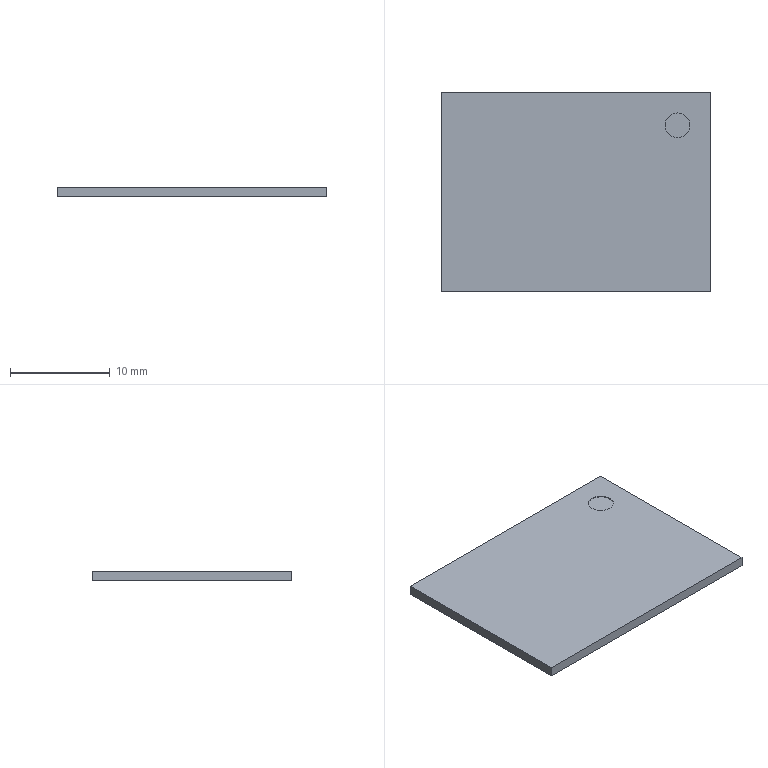Part | STEP file | RJ-USIO-V1_2-220411_183 | 1 solid | 9 faces | box 27 x 20 x 1 mm | volume 539.509 mm3 | plane 7 | cylinder 2 | commonest cylinder face diameters 2.5 x2
STEP:
#1=CARTESIAN_POINT('',(0.,0.,0.));
#2=DIRECTION('',(0.,0.,1.));
#3=DIRECTION('',(1.,0.,0.));
#4=AXIS2_PLACEMENT_3D('',#1,#2,#3);
#5=CARTESIAN_POINT('',(23.867,58.417,0.9));
#6=VERTEX_POINT('',#5);
#7=CARTESIAN_POINT('',(23.867,55.917,0.9));
#8=VERTEX_POINT('',#7);
#9=CARTESIAN_POINT('',(23.867,57.167,0.9));
#10=DIRECTION('',(0.,0.,1.));
#11=DIRECTION('',(-0.000000012,1.,0.));
#12=AXIS2_PLACEMENT_3D('',#9,#10,#11);
#13=CIRCLE('',#12,1.25);
#14=CARTESIAN_POINT('',(23.867,57.167,0.9));
#15=DIRECTION('',(0.,0.,1.));
#16=DIRECTION('',(-0.000000012,1.,0.));
#17=AXIS2_PLACEMENT_3D('',#14,#15,#16);
#18=CYLINDRICAL_SURFACE('',#17,1.25);
#19=CARTESIAN_POINT('',(0.,0.));
#20=DIRECTION('',(1.,0.));
#21=VECTOR('',#20,1.);
#22=LINE('',#19,#21);
#23=(GEOMETRIC_REPRESENTATION_CONTEXT(2)PARAMETRIC_REPRESENTATION_CONTEXT()REPRESENTATION_CONTEXT('',''));
#24=DEFINITIONAL_REPRESENTATION('',(#22),#23);
#25=PCURVE('',#18,#24);
#26=CARTESIAN_POINT('',(23.867,57.167,0.9));
#27=DIRECTION('',(0.,0.,1.));
#28=DIRECTION('',(-0.000000012,1.,0.));
#29=AXIS2_PLACEMENT_3D('',#26,#27,#28);
#30=PLANE('',#29);
#31=CARTESIAN_POINT('',(0.,0.));
#32=DIRECTION('',(1.,0.));
#33=AXIS2_PLACEMENT_2D('',#31,#32);
#34=CIRCLE('',#33,1.25);
#35=(GEOMETRIC_REPRESENTATION_CONTEXT(2)PARAMETRIC_REPRESENTATION_CONTEXT()REPRESENTATION_CONTEXT('',''));
#36=DEFINITIONAL_REPRESENTATION('',(#34),#35);
#37=PCURVE('',#30,#36);
#38=SURFACE_CURVE('',#13,(#25,#37),.PCURVE_S1.);
#39=EDGE_CURVE('',#6,#8,#38,.T.);
#40=ORIENTED_EDGE('',*,*,#39,.T.);
#41=CARTESIAN_POINT('',(23.867,55.917,1.));
#42=VERTEX_POINT('',#41);
#43=CARTESIAN_POINT('',(23.867,55.917,0.9));
#44=DIRECTION('',(0.,0.,1.));
#45=VECTOR('',#44,1.);
#46=LINE('',#43,#45);
#47=CARTESIAN_POINT('',(3.142,0.));
#48=DIRECTION('',(0.,1.));
#49=VECTOR('',#48,1.);
#50=LINE('',#47,#49);
#51=(GEOMETRIC_REPRESENTATION_CONTEXT(2)PARAMETRIC_REPRESENTATION_CONTEXT()REPRESENTATION_CONTEXT('',''));
#52=DEFINITIONAL_REPRESENTATION('',(#50),#51);
#53=PCURVE('',#18,#52);
#54=CARTESIAN_POINT('',(23.867,57.167,0.9));
#55=DIRECTION('',(0.,0.,1.));
#56=DIRECTION('',(-0.000000012,1.,0.));
#57=AXIS2_PLACEMENT_3D('',#54,#55,#56);
#58=CYLINDRICAL_SURFACE('',#57,1.25);
#59=CARTESIAN_POINT('',(3.142,0.));
#60=DIRECTION('',(0.,1.));
#61=VECTOR('',#60,1.);
#62=LINE('',#59,#61);
#63=(GEOMETRIC_REPRESENTATION_CONTEXT(2)PARAMETRIC_REPRESENTATION_CONTEXT()REPRESENTATION_CONTEXT('',''));
#64=DEFINITIONAL_REPRESENTATION('',(#62),#63);
#65=PCURVE('',#58,#64);
#66=SURFACE_CURVE('',#46,(#53,#65),.PCURVE_S1.);
#67=EDGE_CURVE('',#8,#42,#66,.T.);
#68=ORIENTED_EDGE('',*,*,#67,.T.);
#69=CARTESIAN_POINT('',(23.867,58.417,1.));
#70=VERTEX_POINT('',#69);
#71=CARTESIAN_POINT('',(23.867,57.167,1.));
#72=DIRECTION('',(0.,0.,-1.));
#73=DIRECTION('',(0.000000012,-1.,0.));
#74=AXIS2_PLACEMENT_3D('',#71,#72,#73);
#75=CIRCLE('',#74,1.25);
#76=CARTESIAN_POINT('',(3.142,0.1));
#77=DIRECTION('',(-1.,0.));
#78=VECTOR('',#77,1.);
#79=LINE('',#76,#78);
#80=(GEOMETRIC_REPRESENTATION_CONTEXT(2)PARAMETRIC_REPRESENTATION_CONTEXT()REPRESENTATION_CONTEXT('',''));
#81=DEFINITIONAL_REPRESENTATION('',(#79),#80);
#82=PCURVE('',#18,#81);
#83=CARTESIAN_POINT('',(0.2,60.5,1.));
#84=DIRECTION('',(0.,0.,1.));
#85=DIRECTION('',(-0.000000012,1.,0.));
#86=AXIS2_PLACEMENT_3D('',#83,#84,#85);
#87=PLANE('',#86);
#88=CARTESIAN_POINT('',(-4.583,-23.667));
#89=CARTESIAN_POINT('',(-4.583,-21.502));
#90=CARTESIAN_POINT('',(-2.708,-22.584));
#91=CARTESIAN_POINT('',(-0.8333,-23.667));
#92=CARTESIAN_POINT('',(-2.708,-24.749));
#93=CARTESIAN_POINT('',(-4.583,-25.832));
#94=CARTESIAN_POINT('',(-4.583,-23.667));
#95=(BOUNDED_CURVE()B_SPLINE_CURVE(2,(#88,#89,#90,#91,#92,#93,#94),.UNSPECIFIED.,.T.,.F.)B_SPLINE_CURVE_WITH_KNOTS((1,2,2,2,2,1),(-2.094,0.,2.094,4.189,6.283,8.378),.UNSPECIFIED.)CURVE()GEOMETRIC_REPRESENTATION_ITEM()RATIONAL_B_SPLINE_CURVE((1.,0.5,1.,0.5,1.,0.5,1.))REPRESENTATION_ITEM(''));
#96=(GEOMETRIC_REPRESENTATION_CONTEXT(2)PARAMETRIC_REPRESENTATION_CONTEXT()REPRESENTATION_CONTEXT('',''));
#97=DEFINITIONAL_REPRESENTATION('',(#95),#96);
#98=PCURVE('',#87,#97);
#99=SURFACE_CURVE('',#75,(#82,#98),.PCURVE_S1.);
#100=EDGE_CURVE('',#42,#70,#99,.T.);
#101=ORIENTED_EDGE('',*,*,#100,.T.);
#102=CARTESIAN_POINT('',(23.867,58.417,0.9));
#103=DIRECTION('',(0.,0.,1.));
#104=VECTOR('',#103,1.);
#105=LINE('',#102,#104);
#106=CARTESIAN_POINT('',(0.,0.));
#107=DIRECTION('',(0.,1.));
#108=VECTOR('',#107,1.);
#109=LINE('',#106,#108);
#110=(GEOMETRIC_REPRESENTATION_CONTEXT(2)PARAMETRIC_REPRESENTATION_CONTEXT()REPRESENTATION_CONTEXT('',''));
#111=DEFINITIONAL_REPRESENTATION('',(#109),#110);
#112=PCURVE('',#18,#111);
#113=CARTESIAN_POINT('',(6.283,0.));
#114=DIRECTION('',(0.,1.));
#115=VECTOR('',#114,1.);
#116=LINE('',#113,#115);
#117=(GEOMETRIC_REPRESENTATION_CONTEXT(2)PARAMETRIC_REPRESENTATION_CONTEXT()REPRESENTATION_CONTEXT('',''));
#118=DEFINITIONAL_REPRESENTATION('',(#116),#117);
#119=PCURVE('',#58,#118);
#120=SURFACE_CURVE('',#105,(#112,#119),.PCURVE_S1.);
#121=EDGE_CURVE('',#6,#70,#120,.T.);
#122=ORIENTED_EDGE('',*,*,#121,.F.);
#123=EDGE_LOOP('',(#40,#68,#101,#122));
#124=FACE_BOUND('',#123,.F.);
#125=ADVANCED_FACE('',(#124),#18,.F.);
#126=CARTESIAN_POINT('',(23.867,57.167,0.9));
#127=DIRECTION('',(0.,0.,1.));
#128=DIRECTION('',(0.000000012,-1.,0.));
#129=AXIS2_PLACEMENT_3D('',#126,#127,#128);
#130=CIRCLE('',#129,1.25);
#131=CARTESIAN_POINT('',(0.,0.));
#132=DIRECTION('',(-1.,0.));
#133=AXIS2_PLACEMENT_2D('',#131,#132);
#134=CIRCLE('',#133,1.25);
#135=(GEOMETRIC_REPRESENTATION_CONTEXT(2)PARAMETRIC_REPRESENTATION_CONTEXT()REPRESENTATION_CONTEXT('',''));
#136=DEFINITIONAL_REPRESENTATION('',(#134),#135);
#137=PCURVE('',#30,#136);
#138=CARTESIAN_POINT('',(3.142,0.));
#139=DIRECTION('',(1.,0.));
#140=VECTOR('',#139,1.);
#141=LINE('',#138,#140);
#142=(GEOMETRIC_REPRESENTATION_CONTEXT(2)PARAMETRIC_REPRESENTATION_CONTEXT()REPRESENTATION_CONTEXT('',''));
#143=DEFINITIONAL_REPRESENTATION('',(#141),#142);
#144=PCURVE('',#58,#143);
#145=SURFACE_CURVE('',#130,(#137,#144),.PCURVE_S1.);
#146=EDGE_CURVE('',#8,#6,#145,.T.);
#147=ORIENTED_EDGE('',*,*,#146,.F.);
#148=ORIENTED_EDGE('',*,*,#39,.F.);
#149=EDGE_LOOP('',(#147,#148));
#150=FACE_BOUND('',#149,.F.);
#151=ADVANCED_FACE('',(#150),#30,.T.);
#152=ORIENTED_EDGE('',*,*,#121,.T.);
#153=CARTESIAN_POINT('',(23.867,57.167,1.));
#154=DIRECTION('',(0.,0.,-1.));
#155=DIRECTION('',(-0.000000012,1.,0.));
#156=AXIS2_PLACEMENT_3D('',#153,#154,#155);
#157=CIRCLE('',#156,1.25);
#158=CARTESIAN_POINT('',(6.283,0.1));
#159=DIRECTION('',(-1.,0.));
#160=VECTOR('',#159,1.);
#161=LINE('',#158,#160);
#162=(GEOMETRIC_REPRESENTATION_CONTEXT(2)PARAMETRIC_REPRESENTATION_CONTEXT()REPRESENTATION_CONTEXT('',''));
#163=DEFINITIONAL_REPRESENTATION('',(#161),#162);
#164=PCURVE('',#58,#163);
#165=CARTESIAN_POINT('',(-2.083,-23.667));
#166=CARTESIAN_POINT('',(-2.083,-25.832));
#167=CARTESIAN_POINT('',(-3.958,-24.749));
#168=CARTESIAN_POINT('',(-5.833,-23.667));
#169=CARTESIAN_POINT('',(-3.958,-22.584));
#170=CARTESIAN_POINT('',(-2.083,-21.502));
#171=CARTESIAN_POINT('',(-2.083,-23.667));
#172=(BOUNDED_CURVE()B_SPLINE_CURVE(2,(#165,#166,#167,#168,#169,#170,#171),.UNSPECIFIED.,.T.,.F.)B_SPLINE_CURVE_WITH_KNOTS((1,2,2,2,2,1),(-2.094,0.,2.094,4.189,6.283,8.378),.UNSPECIFIED.)CURVE()GEOMETRIC_REPRESENTATION_ITEM()RATIONAL_B_SPLINE_CURVE((1.,0.5,1.,0.5,1.,0.5,1.))REPRESENTATION_ITEM(''));
#173=(GEOMETRIC_REPRESENTATION_CONTEXT(2)PARAMETRIC_REPRESENTATION_CONTEXT()REPRESENTATION_CONTEXT('',''));
#174=DEFINITIONAL_REPRESENTATION('',(#172),#173);
#175=PCURVE('',#87,#174);
#176=SURFACE_CURVE('',#157,(#164,#175),.PCURVE_S1.);
#177=EDGE_CURVE('',#70,#42,#176,.T.);
#178=ORIENTED_EDGE('',*,*,#177,.T.);
#179=ORIENTED_EDGE('',*,*,#67,.F.);
#180=ORIENTED_EDGE('',*,*,#146,.T.);
#181=EDGE_LOOP('',(#152,#178,#179,#180));
#182=FACE_BOUND('',#181,.F.);
#183=ADVANCED_FACE('',(#182),#58,.F.);
#184=CARTESIAN_POINT('',(27.2,60.5,1.));
#185=VERTEX_POINT('',#184);
#186=CARTESIAN_POINT('',(0.2,60.5,1.));
#187=VERTEX_POINT('',#186);
#188=CARTESIAN_POINT('',(27.2,60.5,1.));
#189=DIRECTION('',(-1.,-0.000000012,0.));
#190=VECTOR('',#189,1.);
#191=LINE('',#188,#190);
#192=CARTESIAN_POINT('',(0.,-27.));
#193=DIRECTION('',(0.,1.));
#194=VECTOR('',#193,1.);
#195=LINE('',#192,#194);
#196=(GEOMETRIC_REPRESENTATION_CONTEXT(2)PARAMETRIC_REPRESENTATION_CONTEXT()REPRESENTATION_CONTEXT('',''));
#197=DEFINITIONAL_REPRESENTATION('',(#195),#196);
#198=PCURVE('',#87,#197);
#199=CARTESIAN_POINT('',(0.2,60.5,0.));
#200=DIRECTION('',(0.000000012,-1.,0.));
#201=DIRECTION('',(0.,0.,-1.));
#202=AXIS2_PLACEMENT_3D('',#199,#200,#201);
#203=PLANE('',#202);
#204=CARTESIAN_POINT('',(-1.,27.));
#205=DIRECTION('',(0.,-1.));
#206=VECTOR('',#205,1.);
#207=LINE('',#204,#206);
#208=(GEOMETRIC_REPRESENTATION_CONTEXT(2)PARAMETRIC_REPRESENTATION_CONTEXT()REPRESENTATION_CONTEXT('',''));
#209=DEFINITIONAL_REPRESENTATION('',(#207),#208);
#210=PCURVE('',#203,#209);
#211=SURFACE_CURVE('',#191,(#198,#210),.PCURVE_S1.);
#212=EDGE_CURVE('',#185,#187,#211,.T.);
#213=ORIENTED_EDGE('',*,*,#212,.F.);
#214=CARTESIAN_POINT('',(27.2,40.5,1.));
#215=VERTEX_POINT('',#214);
#216=CARTESIAN_POINT('',(27.2,40.5,1.));
#217=DIRECTION('',(-0.000000012,1.,0.));
#218=VECTOR('',#217,1.);
#219=LINE('',#216,#218);
#220=CARTESIAN_POINT('',(-20.,-27.));
#221=DIRECTION('',(1.,0.));
#222=VECTOR('',#221,1.);
#223=LINE('',#220,#222);
#224=(GEOMETRIC_REPRESENTATION_CONTEXT(2)PARAMETRIC_REPRESENTATION_CONTEXT()REPRESENTATION_CONTEXT('',''));
#225=DEFINITIONAL_REPRESENTATION('',(#223),#224);
#226=PCURVE('',#87,#225);
#227=CARTESIAN_POINT('',(27.2,60.5,0.));
#228=DIRECTION('',(1.,0.000000012,0.));
#229=DIRECTION('',(0.,0.,-1.));
#230=AXIS2_PLACEMENT_3D('',#227,#228,#229);
#231=PLANE('',#230);
#232=CARTESIAN_POINT('',(-1.,-20.));
#233=DIRECTION('',(0.,1.));
#234=VECTOR('',#233,1.);
#235=LINE('',#232,#234);
#236=(GEOMETRIC_REPRESENTATION_CONTEXT(2)PARAMETRIC_REPRESENTATION_CONTEXT()REPRESENTATION_CONTEXT('',''));
#237=DEFINITIONAL_REPRESENTATION('',(#235),#236);
#238=PCURVE('',#231,#237);
#239=SURFACE_CURVE('',#219,(#226,#238),.PCURVE_S1.);
#240=EDGE_CURVE('',#215,#185,#239,.T.);
#241=ORIENTED_EDGE('',*,*,#240,.F.);
#242=CARTESIAN_POINT('',(0.2,40.5,1.));
#243=VERTEX_POINT('',#242);
#244=CARTESIAN_POINT('',(27.2,40.5,1.));
#245=DIRECTION('',(-1.,-0.000000012,0.));
#246=VECTOR('',#245,1.);
#247=LINE('',#244,#246);
#248=CARTESIAN_POINT('',(-20.,-27.));
#249=DIRECTION('',(0.,1.));
#250=VECTOR('',#249,1.);
#251=LINE('',#248,#250);
#252=(GEOMETRIC_REPRESENTATION_CONTEXT(2)PARAMETRIC_REPRESENTATION_CONTEXT()REPRESENTATION_CONTEXT('',''));
#253=DEFINITIONAL_REPRESENTATION('',(#251),#252);
#254=PCURVE('',#87,#253);
#255=CARTESIAN_POINT('',(0.2,40.5,0.));
#256=DIRECTION('',(0.000000012,-1.,0.));
#257=DIRECTION('',(0.,0.,-1.));
#258=AXIS2_PLACEMENT_3D('',#255,#256,#257);
#259=PLANE('',#258);
#260=CARTESIAN_POINT('',(-1.,27.));
#261=DIRECTION('',(0.,-1.));
#262=VECTOR('',#261,1.);
#263=LINE('',#260,#262);
#264=(GEOMETRIC_REPRESENTATION_CONTEXT(2)PARAMETRIC_REPRESENTATION_CONTEXT()REPRESENTATION_CONTEXT('',''));
#265=DEFINITIONAL_REPRESENTATION('',(#263),#264);
#266=PCURVE('',#259,#265);
#267=SURFACE_CURVE('',#247,(#254,#266),.PCURVE_S1.);
#268=EDGE_CURVE('',#215,#243,#267,.T.);
#269=ORIENTED_EDGE('',*,*,#268,.T.);
#270=CARTESIAN_POINT('',(0.2,40.5,1.));
#271=DIRECTION('',(-0.000000012,1.,0.));
#272=VECTOR('',#271,1.);
#273=LINE('',#270,#272);
#274=CARTESIAN_POINT('',(-20.,0.));
#275=DIRECTION('',(1.,0.));
#276=VECTOR('',#275,1.);
#277=LINE('',#274,#276);
#278=(GEOMETRIC_REPRESENTATION_CONTEXT(2)PARAMETRIC_REPRESENTATION_CONTEXT()REPRESENTATION_CONTEXT('',''));
#279=DEFINITIONAL_REPRESENTATION('',(#277),#278);
#280=PCURVE('',#87,#279);
#281=CARTESIAN_POINT('',(0.2,60.5,0.));
#282=DIRECTION('',(1.,0.000000012,0.));
#283=DIRECTION('',(0.,0.,-1.));
#284=AXIS2_PLACEMENT_3D('',#281,#282,#283);
#285=PLANE('',#284);
#286=CARTESIAN_POINT('',(-1.,-20.));
#287=DIRECTION('',(0.,1.));
#288=VECTOR('',#287,1.);
#289=LINE('',#286,#288);
#290=(GEOMETRIC_REPRESENTATION_CONTEXT(2)PARAMETRIC_REPRESENTATION_CONTEXT()REPRESENTATION_CONTEXT('',''));
#291=DEFINITIONAL_REPRESENTATION('',(#289),#290);
#292=PCURVE('',#285,#291);
#293=SURFACE_CURVE('',#273,(#280,#292),.PCURVE_S1.);
#294=EDGE_CURVE('',#243,#187,#293,.T.);
#295=ORIENTED_EDGE('',*,*,#294,.T.);
#296=EDGE_LOOP('',(#213,#241,#269,#295));
#297=FACE_BOUND('',#296,.F.);
#298=ORIENTED_EDGE('',*,*,#177,.F.);
#299=ORIENTED_EDGE('',*,*,#100,.F.);
#300=EDGE_LOOP('',(#298,#299));
#301=FACE_BOUND('',#300,.F.);
#302=ADVANCED_FACE('',(#297,#301),#87,.T.);
#303=ORIENTED_EDGE('',*,*,#212,.T.);
#304=CARTESIAN_POINT('',(0.2,60.5,0.));
#305=VERTEX_POINT('',#304);
#306=CARTESIAN_POINT('',(0.2,60.5,1.));
#307=DIRECTION('',(0.,0.,-1.));
#308=VECTOR('',#307,1.);
#309=LINE('',#306,#308);
#310=CARTESIAN_POINT('',(-1.,0.));
#311=DIRECTION('',(1.,0.));
#312=VECTOR('',#311,1.);
#313=LINE('',#310,#312);
#314=(GEOMETRIC_REPRESENTATION_CONTEXT(2)PARAMETRIC_REPRESENTATION_CONTEXT()REPRESENTATION_CONTEXT('',''));
#315=DEFINITIONAL_REPRESENTATION('',(#313),#314);
#316=PCURVE('',#203,#315);
#317=CARTESIAN_POINT('',(-1.,0.));
#318=DIRECTION('',(1.,0.));
#319=VECTOR('',#318,1.);
#320=LINE('',#317,#319);
#321=(GEOMETRIC_REPRESENTATION_CONTEXT(2)PARAMETRIC_REPRESENTATION_CONTEXT()REPRESENTATION_CONTEXT('',''));
#322=DEFINITIONAL_REPRESENTATION('',(#320),#321);
#323=PCURVE('',#285,#322);
#324=SURFACE_CURVE('',#309,(#316,#323),.PCURVE_S1.);
#325=EDGE_CURVE('',#187,#305,#324,.T.);
#326=ORIENTED_EDGE('',*,*,#325,.T.);
#327=CARTESIAN_POINT('',(27.2,60.5,0.));
#328=VERTEX_POINT('',#327);
#329=CARTESIAN_POINT('',(27.2,60.5,0.));
#330=DIRECTION('',(-1.,-0.000000012,0.));
#331=VECTOR('',#330,1.);
#332=LINE('',#329,#331);
#333=CARTESIAN_POINT('',(0.,27.));
#334=DIRECTION('',(0.,-1.));
#335=VECTOR('',#334,1.);
#336=LINE('',#333,#335);
#337=(GEOMETRIC_REPRESENTATION_CONTEXT(2)PARAMETRIC_REPRESENTATION_CONTEXT()REPRESENTATION_CONTEXT('',''));
#338=DEFINITIONAL_REPRESENTATION('',(#336),#337);
#339=PCURVE('',#203,#338);
#340=CARTESIAN_POINT('',(0.2,60.5,0.));
#341=DIRECTION('',(0.,0.,1.));
#342=DIRECTION('',(-0.000000012,1.,0.));
#343=AXIS2_PLACEMENT_3D('',#340,#341,#342);
#344=PLANE('',#343);
#345=CARTESIAN_POINT('',(0.,-27.));
#346=DIRECTION('',(0.,1.));
#347=VECTOR('',#346,1.);
#348=LINE('',#345,#347);
#349=(GEOMETRIC_REPRESENTATION_CONTEXT(2)PARAMETRIC_REPRESENTATION_CONTEXT()REPRESENTATION_CONTEXT('',''));
#350=DEFINITIONAL_REPRESENTATION('',(#348),#349);
#351=PCURVE('',#344,#350);
#352=SURFACE_CURVE('',#332,(#339,#351),.PCURVE_S1.);
#353=EDGE_CURVE('',#328,#305,#352,.T.);
#354=ORIENTED_EDGE('',*,*,#353,.F.);
#355=CARTESIAN_POINT('',(27.2,60.5,1.));
#356=DIRECTION('',(0.,0.,-1.));
#357=VECTOR('',#356,1.);
#358=LINE('',#355,#357);
#359=CARTESIAN_POINT('',(-1.,27.));
#360=DIRECTION('',(1.,0.));
#361=VECTOR('',#360,1.);
#362=LINE('',#359,#361);
#363=(GEOMETRIC_REPRESENTATION_CONTEXT(2)PARAMETRIC_REPRESENTATION_CONTEXT()REPRESENTATION_CONTEXT('',''));
#364=DEFINITIONAL_REPRESENTATION('',(#362),#363);
#365=PCURVE('',#203,#364);
#366=CARTESIAN_POINT('',(-1.,0.));
#367=DIRECTION('',(1.,0.));
#368=VECTOR('',#367,1.);
#369=LINE('',#366,#368);
#370=(GEOMETRIC_REPRESENTATION_CONTEXT(2)PARAMETRIC_REPRESENTATION_CONTEXT()REPRESENTATION_CONTEXT('',''));
#371=DEFINITIONAL_REPRESENTATION('',(#369),#370);
#372=PCURVE('',#231,#371);
#373=SURFACE_CURVE('',#358,(#365,#372),.PCURVE_S1.);
#374=EDGE_CURVE('',#185,#328,#373,.T.);
#375=ORIENTED_EDGE('',*,*,#374,.F.);
#376=EDGE_LOOP('',(#303,#326,#354,#375));
#377=FACE_BOUND('',#376,.F.);
#378=ADVANCED_FACE('',(#377),#203,.F.);
#379=CARTESIAN_POINT('',(0.2,40.5,0.));
#380=VERTEX_POINT('',#379);
#381=CARTESIAN_POINT('',(0.2,40.5,1.));
#382=DIRECTION('',(0.,0.,-1.));
#383=VECTOR('',#382,1.);
#384=LINE('',#381,#383);
#385=CARTESIAN_POINT('',(-1.,-20.));
#386=DIRECTION('',(1.,0.));
#387=VECTOR('',#386,1.);
#388=LINE('',#385,#387);
#389=(GEOMETRIC_REPRESENTATION_CONTEXT(2)PARAMETRIC_REPRESENTATION_CONTEXT()REPRESENTATION_CONTEXT('',''));
#390=DEFINITIONAL_REPRESENTATION('',(#388),#389);
#391=PCURVE('',#285,#390);
#392=CARTESIAN_POINT('',(-1.,0.));
#393=DIRECTION('',(1.,0.));
#394=VECTOR('',#393,1.);
#395=LINE('',#392,#394);
#396=(GEOMETRIC_REPRESENTATION_CONTEXT(2)PARAMETRIC_REPRESENTATION_CONTEXT()REPRESENTATION_CONTEXT('',''));
#397=DEFINITIONAL_REPRESENTATION('',(#395),#396);
#398=PCURVE('',#259,#397);
#399=SURFACE_CURVE('',#384,(#391,#398),.PCURVE_S1.);
#400=EDGE_CURVE('',#243,#380,#399,.T.);
#401=ORIENTED_EDGE('',*,*,#400,.T.);
#402=CARTESIAN_POINT('',(0.2,40.5,0.));
#403=DIRECTION('',(-0.000000012,1.,0.));
#404=VECTOR('',#403,1.);
#405=LINE('',#402,#404);
#406=CARTESIAN_POINT('',(0.,-20.));
#407=DIRECTION('',(0.,1.));
#408=VECTOR('',#407,1.);
#409=LINE('',#406,#408);
#410=(GEOMETRIC_REPRESENTATION_CONTEXT(2)PARAMETRIC_REPRESENTATION_CONTEXT()REPRESENTATION_CONTEXT('',''));
#411=DEFINITIONAL_REPRESENTATION('',(#409),#410);
#412=PCURVE('',#285,#411);
#413=CARTESIAN_POINT('',(-20.,0.));
#414=DIRECTION('',(1.,0.));
#415=VECTOR('',#414,1.);
#416=LINE('',#413,#415);
#417=(GEOMETRIC_REPRESENTATION_CONTEXT(2)PARAMETRIC_REPRESENTATION_CONTEXT()REPRESENTATION_CONTEXT('',''));
#418=DEFINITIONAL_REPRESENTATION('',(#416),#417);
#419=PCURVE('',#344,#418);
#420=SURFACE_CURVE('',#405,(#412,#419),.PCURVE_S1.);
#421=EDGE_CURVE('',#380,#305,#420,.T.);
#422=ORIENTED_EDGE('',*,*,#421,.T.);
#423=ORIENTED_EDGE('',*,*,#325,.F.);
#424=ORIENTED_EDGE('',*,*,#294,.F.);
#425=EDGE_LOOP('',(#401,#422,#423,#424));
#426=FACE_BOUND('',#425,.F.);
#427=ADVANCED_FACE('',(#426),#285,.F.);
#428=ORIENTED_EDGE('',*,*,#400,.F.);
#429=ORIENTED_EDGE('',*,*,#268,.F.);
#430=CARTESIAN_POINT('',(27.2,40.5,0.));
#431=VERTEX_POINT('',#430);
#432=CARTESIAN_POINT('',(27.2,40.5,1.));
#433=DIRECTION('',(0.,0.,-1.));
#434=VECTOR('',#433,1.);
#435=LINE('',#432,#434);
#436=CARTESIAN_POINT('',(-1.,27.));
#437=DIRECTION('',(1.,0.));
#438=VECTOR('',#437,1.);
#439=LINE('',#436,#438);
#440=(GEOMETRIC_REPRESENTATION_CONTEXT(2)PARAMETRIC_REPRESENTATION_CONTEXT()REPRESENTATION_CONTEXT('',''));
#441=DEFINITIONAL_REPRESENTATION('',(#439),#440);
#442=PCURVE('',#259,#441);
#443=CARTESIAN_POINT('',(-1.,-20.));
#444=DIRECTION('',(1.,0.));
#445=VECTOR('',#444,1.);
#446=LINE('',#443,#445);
#447=(GEOMETRIC_REPRESENTATION_CONTEXT(2)PARAMETRIC_REPRESENTATION_CONTEXT()REPRESENTATION_CONTEXT('',''));
#448=DEFINITIONAL_REPRESENTATION('',(#446),#447);
#449=PCURVE('',#231,#448);
#450=SURFACE_CURVE('',#435,(#442,#449),.PCURVE_S1.);
#451=EDGE_CURVE('',#215,#431,#450,.T.);
#452=ORIENTED_EDGE('',*,*,#451,.T.);
#453=CARTESIAN_POINT('',(27.2,40.5,0.));
#454=DIRECTION('',(-1.,-0.000000012,0.));
#455=VECTOR('',#454,1.);
#456=LINE('',#453,#455);
#457=CARTESIAN_POINT('',(0.,27.));
#458=DIRECTION('',(0.,-1.));
#459=VECTOR('',#458,1.);
#460=LINE('',#457,#459);
#461=(GEOMETRIC_REPRESENTATION_CONTEXT(2)PARAMETRIC_REPRESENTATION_CONTEXT()REPRESENTATION_CONTEXT('',''));
#462=DEFINITIONAL_REPRESENTATION('',(#460),#461);
#463=PCURVE('',#259,#462);
#464=CARTESIAN_POINT('',(-20.,-27.));
#465=DIRECTION('',(0.,1.));
#466=VECTOR('',#465,1.);
#467=LINE('',#464,#466);
#468=(GEOMETRIC_REPRESENTATION_CONTEXT(2)PARAMETRIC_REPRESENTATION_CONTEXT()REPRESENTATION_CONTEXT('',''));
#469=DEFINITIONAL_REPRESENTATION('',(#467),#468);
#470=PCURVE('',#344,#469);
#471=SURFACE_CURVE('',#456,(#463,#470),.PCURVE_S1.);
#472=EDGE_CURVE('',#431,#380,#471,.T.);
#473=ORIENTED_EDGE('',*,*,#472,.T.);
#474=EDGE_LOOP('',(#428,#429,#452,#473));
#475=FACE_BOUND('',#474,.F.);
#476=ADVANCED_FACE('',(#475),#259,.T.);
#477=CARTESIAN_POINT('',(27.2,40.5,0.));
#478=DIRECTION('',(-0.000000012,1.,0.));
#479=VECTOR('',#478,1.);
#480=LINE('',#477,#479);
#481=CARTESIAN_POINT('',(0.,-20.));
#482=DIRECTION('',(0.,1.));
#483=VECTOR('',#482,1.);
#484=LINE('',#481,#483);
#485=(GEOMETRIC_REPRESENTATION_CONTEXT(2)PARAMETRIC_REPRESENTATION_CONTEXT()REPRESENTATION_CONTEXT('',''));
#486=DEFINITIONAL_REPRESENTATION('',(#484),#485);
#487=PCURVE('',#231,#486);
#488=CARTESIAN_POINT('',(-20.,-27.));
#489=DIRECTION('',(1.,0.));
#490=VECTOR('',#489,1.);
#491=LINE('',#488,#490);
#492=(GEOMETRIC_REPRESENTATION_CONTEXT(2)PARAMETRIC_REPRESENTATION_CONTEXT()REPRESENTATION_CONTEXT('',''));
#493=DEFINITIONAL_REPRESENTATION('',(#491),#492);
#494=PCURVE('',#344,#493);
#495=SURFACE_CURVE('',#480,(#487,#494),.PCURVE_S1.);
#496=EDGE_CURVE('',#431,#328,#495,.T.);
#497=ORIENTED_EDGE('',*,*,#496,.F.);
#498=ORIENTED_EDGE('',*,*,#451,.F.);
#499=ORIENTED_EDGE('',*,*,#240,.T.);
#500=ORIENTED_EDGE('',*,*,#374,.T.);
#501=EDGE_LOOP('',(#497,#498,#499,#500));
#502=FACE_BOUND('',#501,.F.);
#503=ADVANCED_FACE('',(#502),#231,.T.);
#504=ORIENTED_EDGE('',*,*,#496,.T.);
#505=ORIENTED_EDGE('',*,*,#353,.T.);
#506=ORIENTED_EDGE('',*,*,#421,.F.);
#507=ORIENTED_EDGE('',*,*,#472,.F.);
#508=EDGE_LOOP('',(#504,#505,#506,#507));
#509=FACE_BOUND('',#508,.F.);
#510=ADVANCED_FACE('',(#509),#344,.F.);
#511=CLOSED_SHELL('',(#125,#151,#183,#302,#378,#427,#476,#503,#510));
#512=MANIFOLD_SOLID_BREP('',#511);
#513=(LENGTH_UNIT()NAMED_UNIT(*)SI_UNIT(.MILLI.,.METRE.));
#514=UNCERTAINTY_MEASURE_WITH_UNIT(LENGTH_MEASURE(0.0000001),#513,'','');
#515=(NAMED_UNIT(*)PLANE_ANGLE_UNIT()SI_UNIT($,.RADIAN.));
#516=(NAMED_UNIT(*)SI_UNIT($,.STERADIAN.)SOLID_ANGLE_UNIT());
#517=(GEOMETRIC_REPRESENTATION_CONTEXT(3)GLOBAL_UNCERTAINTY_ASSIGNED_CONTEXT((#514))GLOBAL_UNIT_ASSIGNED_CONTEXT((#513,#515,#516))REPRESENTATION_CONTEXT('',''));
#518=ADVANCED_BREP_SHAPE_REPRESENTATION('',(#4,#512),#517);